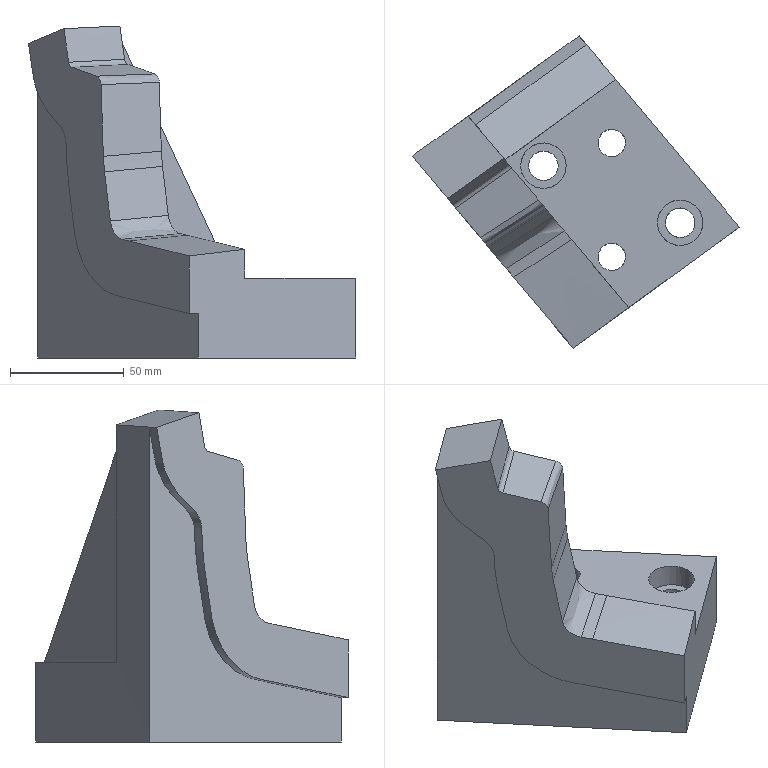Part | NX | features solid 2 | 1 solid | 32 faces | box 143.534 x 137.051 x 145.71 mm | volume 544801 mm3 | spline 15 | plane 11 | cylinder 6 | commonest cylinder face diameters 12 x2 13 x2 20 x2